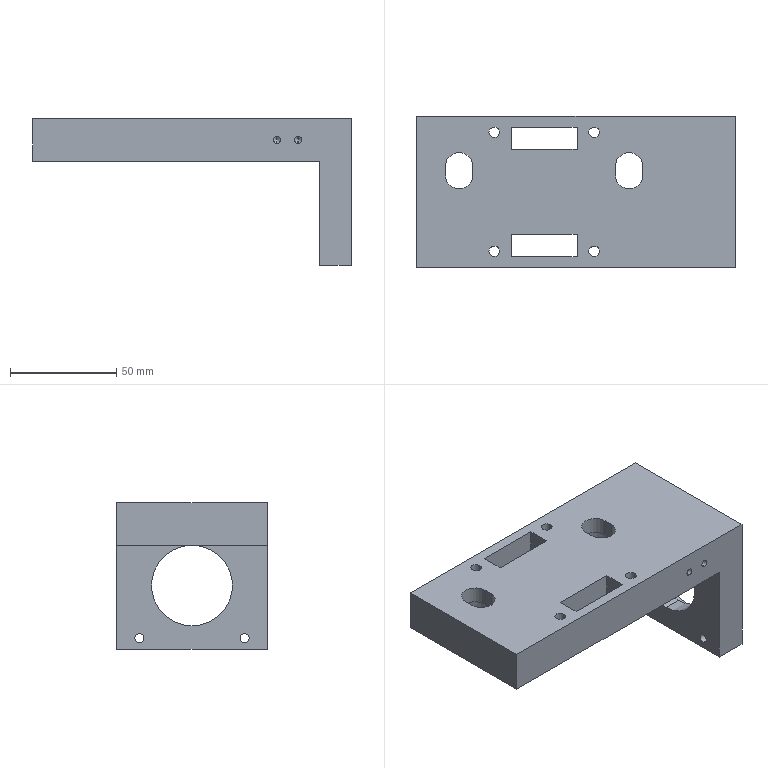Part | 1 solid | 74 faces | box 150 x 71 x 69 mm | volume 204934 mm3 | cylinder 36 | plane 26 | cone 12 | commonest cylinder face diameters 3.3 x8 4.2 x8 5 x8 13 x4 19 x4 38 x2